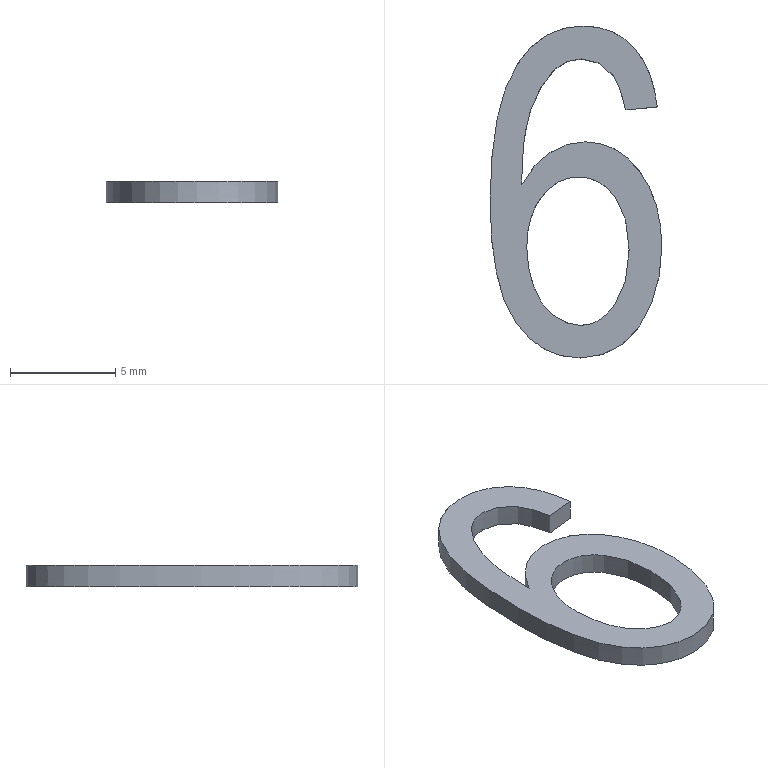Part | STEP file | lll_id1466_x_t | 1 solid | 4 faces | box 8.148 x 15.751 x 1 mm | volume 62.119 mm3 | other 2 | plane 2